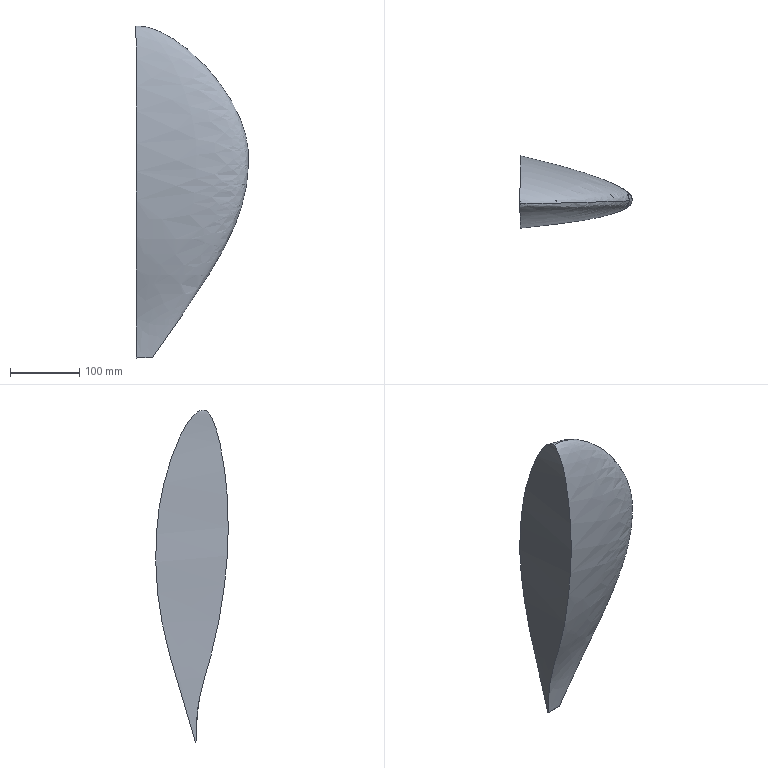Part | SolidWorks | features BaseBody 1 | 1 solid | 4 faces | box 163.209 x 104.812 x 479.995 mm | volume 2908477 mm3 | spline 3 | plane 1